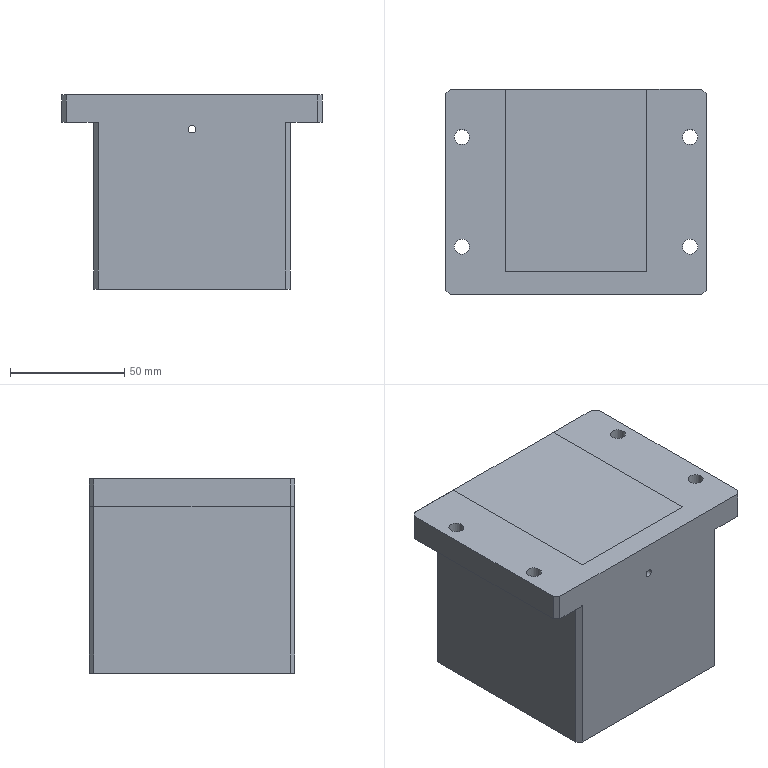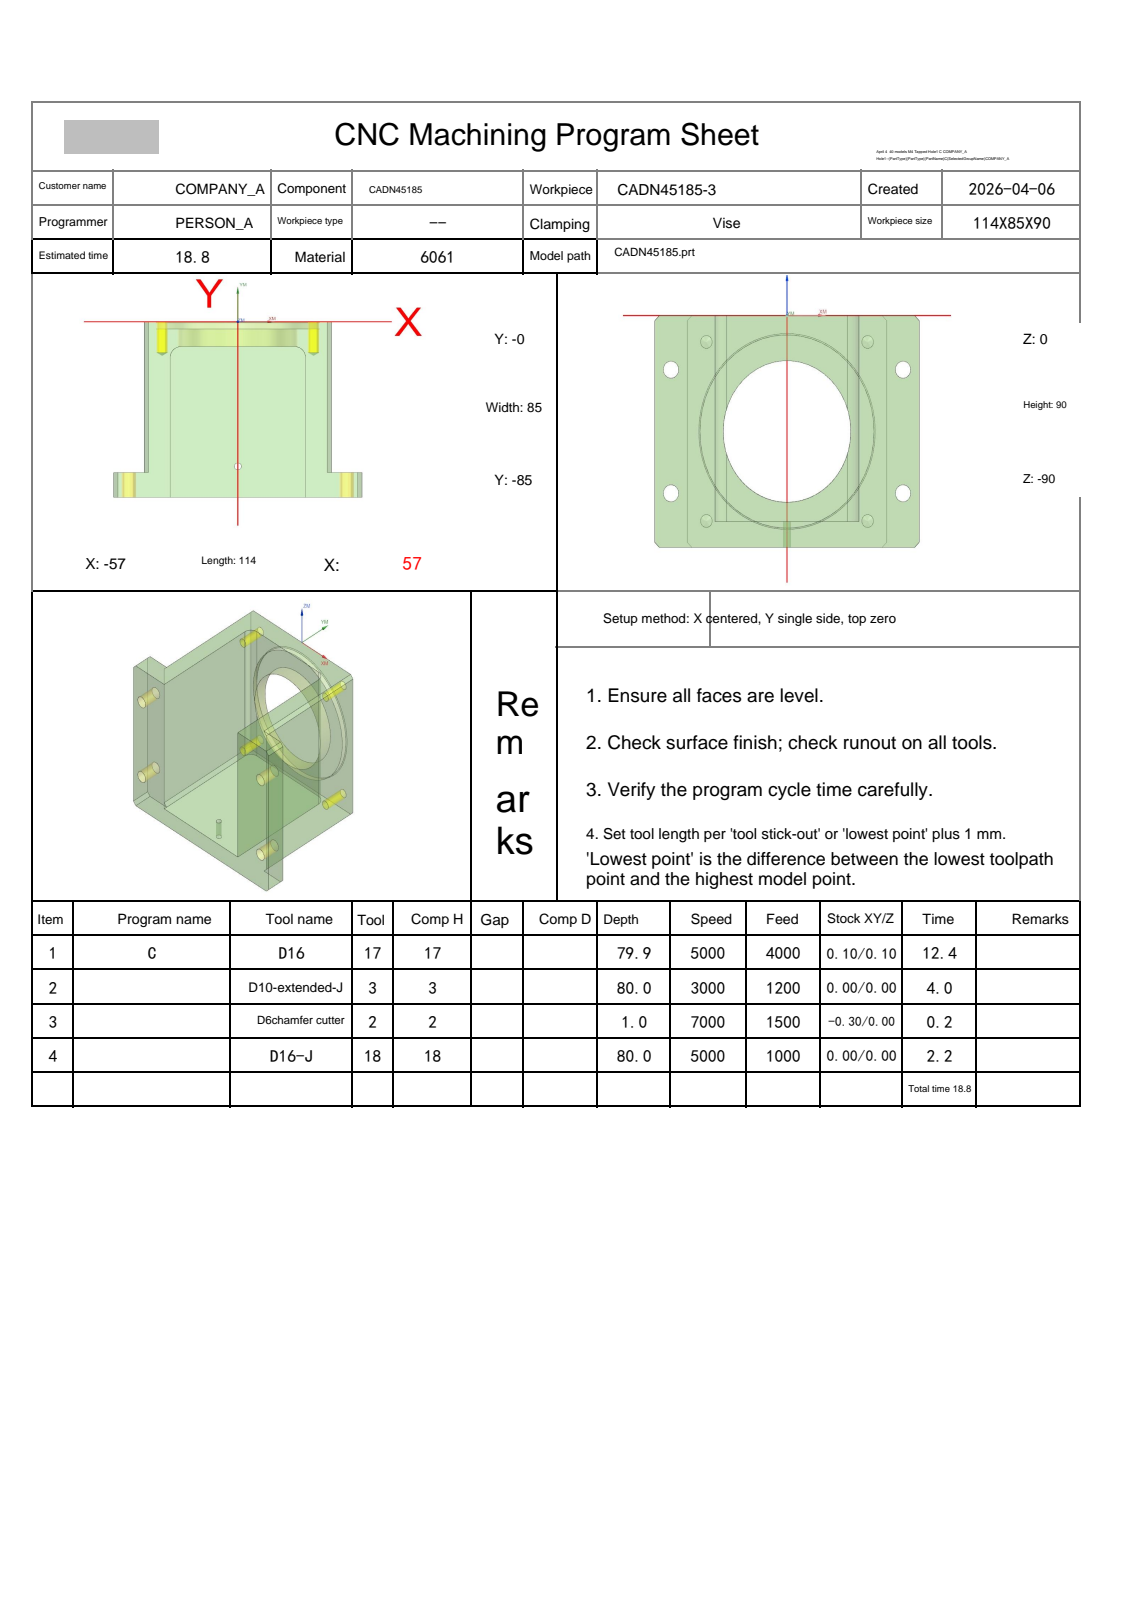NC program | NX | posted by the shop | part box 114 x 90 x 85 mm
Lines 14210 to 14367 of 14367:
N3 T02 M06
(D6chamfer cutter  D=6. R=0. H=02 ce=-0.30 di=0.00)
G00 G90 G54 X30.3 Y-75.384 M03 S7000
G43 H02 Z50.
M08
Z2.5
G01 Y-85. Z-1. F1500.
Y-17.
G03 X26. Y-12.7 I-4.3 J0.0
G01 X-26.
G03 X-30.3 Y-17. I0.0 J-4.3
G01 Y-85.
Z1.5
G00 Z50.
G91 G28 Z0.0
M05
M09
G91 G28 Z0.0
M01
N4 T18 M06
(D16-J  D=16. R=0. H=18 ce=0.40 di=0.00)
G00 G90 G54 X3.4 Y-96.2 M03 S5000
G43 H18 Z10.4
M08
Z-78.5
G01 Z-80. F1000.
Y-89.8
G03 X6.6 Y-86.6 I0.0 J3.2
G01 Y-37.996
G03 X5.004 Y-36.4 I-1.6 J-.004
G01 X-5.004
G03 X-6.6 Y-37.996 I.004 J-1.6
G01 Y-85.
G02 X-8.2 Y-86.6 I-1.6 J0.0
G01 X-13.
G02 X-14.6 Y-85. I0.0 J1.6
G01 Y-29.996
G02 X-13.004 Y-28.4 I1.6 J-.004
G01 X13.004
G02 X14.6 Y-29.996 I-.004 J-1.6
G01 Y-85.361
G03 X15.799 Y-86.91 I1.6 J.001
G01 X20.6 Y-88.149
G03 X21. Y-88.2 I.4 J1.549
X22.6 Y-86.6 I0.0 J1.6
G01 Y-21.997
G03 X21.003 Y-20.4 I-1.6 J-.003
G01 X-21.003
G03 X-22.6 Y-21.997 I.003 J-1.6
G01 Y-86.6
G03 X-19.4 Y-89.8 I3.2 J0.0
G01 Y-96.2
Z-78.5
G00 Z10.4
G00 G90 X19.601 Y-96.2 M03 S5000
Z10.
Z-9.
G01 Z-10. F1000.
G41 D18
X19.801
G03 X23. Y-93. I-.001 J3.2
G01 Y-20.
X-23.
Y-93.
G03 X-19.801 Y-96.2 I3.2 J0.0
G01 G40 X-19.601
Z-9.
G00 X19.601
Z-19.
G01 Z-20.
G41 D18
X19.801
G03 X23. Y-93. I-.001 J3.2
G01 Y-20.
X-23.
Y-93.
G03 X-19.801 Y-96.2 I3.2 J0.0
G01 G40 X-19.601
Z-19.
G00 X19.601
Z-29.
G01 Z-30.
G41 D18
X19.801
G03 X23. Y-93. I-.001 J3.2
G01 Y-20.
X-23.
Y-93.
G03 X-19.801 Y-96.2 I3.2 J0.0
G01 G40 X-19.601
Z-29.
G00 X19.601
Z-39.
G01 Z-40.
G41 D18
X19.801
G03 X23. Y-93. I-.001 J3.2
G01 Y-20.
X-23.
Y-93.
G03 X-19.801 Y-96.2 I3.2 J0.0
G01 G40 X-19.601
Z-39.
G00 X19.601
Z-49.
G01 Z-50.
G41 D18
X19.801
G03 X23. Y-93. I-.001 J3.2
G01 Y-20.
X-23.
Y-93.
G03 X-19.801 Y-96.2 I3.2 J0.0
G01 G40 X-19.601
Z-49.
G00 X19.601
Z-59.
G01 Z-60.
G41 D18
X19.801
G03 X23. Y-93. I-.001 J3.2
G01 Y-20.
X-23.
Y-93.
G03 X-19.801 Y-96.2 I3.2 J0.0
G01 G40 X-19.601
Z-59.
G00 X19.601
Z-69.
G01 Z-70.
G41 D18
X19.801
G03 X23. Y-93. I-.001 J3.2
G01 Y-20.
X-23.
Y-93.
G03 X-19.801 Y-96.2 I3.2 J0.0
G01 G40 X-19.601
Z-69.
G00 X19.601
Z-79.
G01 Z-80.
G41 D18
X19.801
G03 X23. Y-93. I-.001 J3.2
G01 Y-20.
X-23.
Y-93.
G03 X-19.801 Y-96.2 I3.2 J0.0
G01 G40 X-19.601
Z-79.
G00 Z10.
M05
M09
G91 G28 Z0.0
G91 G28 Y0.0
M30
%